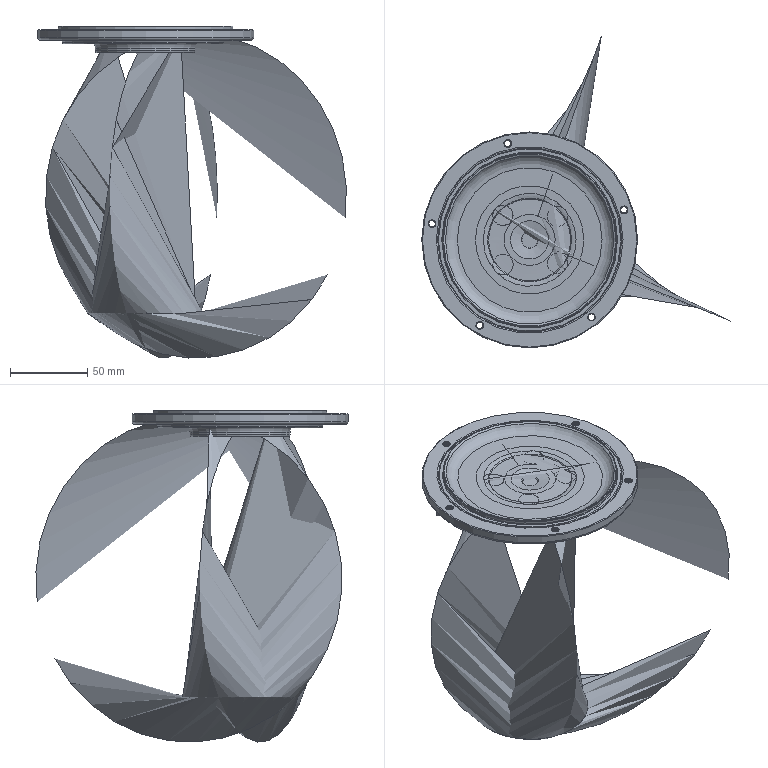NC program | NX | posted with a generic post
Lines 1 to 30 of 33119:
N10 G17 G21 G94 G90
(FLOOR_WALL_1 , TOOL : D10JING)
N12 T11 M6
N14 G54
N16 G17 G0 G90 X-3.981 Y75.27 S9500 M3
N18 G43 Z30. H11
N20 Z-1.35
N22 G94 G1 Z-2.35 F1250.
N24 X-0.866 Y69.875
N26 G3 X0. Y69.375 R1.
N28 G2 X69.375 Y0. R69.375
N30 X0. Y69.375 R-69.375
N32 G1 Y64.375
N34 G2 X64.375 Y0. R64.375
N36 X0. Y64.375 R-64.375
N38 G1 Y62.385
N40 G2 X62.385 Y0. R62.385
N42 X0. Y62.385 R-62.385
N44 G1 X-0.866
N46 G3 X0. Y61.885 R1.
N48 G2 X61.885 Y0. R61.885
N50 X0. Y61.885 R-61.885
N52 G3 X0.866 Y62.385 R1.
N54 G1 X1.434 Y63.369
N56 Z-1.35
N58 G0 Z30.